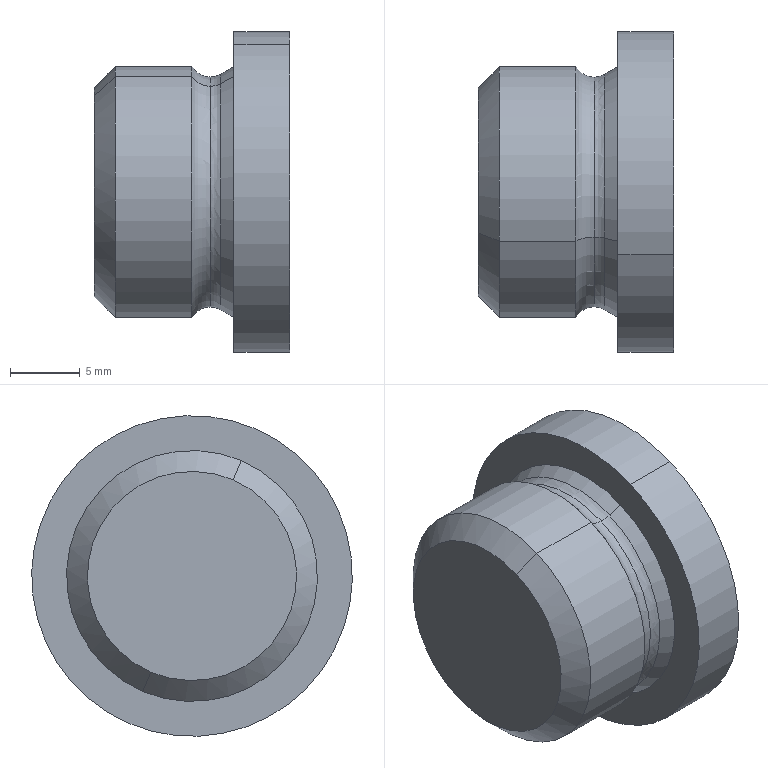Part | SolidWorks | features BaseBody 1 | 1 solid | 34 faces | box 14 x 23 x 23 mm | volume 3610 mm3 | plane 15 | cone 11 | torus 4 | cylinder 4 | commonest cylinder face diameters 18 x2 23 x2
STEP:
#1=CARTESIAN_POINT('',(329.849,223.125,-7.769));
#2=VERTEX_POINT('',#1);
#3=CARTESIAN_POINT('',(329.099,223.046,-7.584));
#4=VERTEX_POINT('',#3);
#5=CARTESIAN_POINT('',(329.099,223.636,-8.963));
#6=DIRECTION('',(0.,-0.9193,-0.3935));
#7=DIRECTION('',(0.,0.3935,-0.9193));
#8=AXIS2_PLACEMENT_3D('',#5,#6,#7);
#9=CIRCLE('',#8,1.5);
#10=EDGE_CURVE('',#2,#4,#9,.T.);
#11=ORIENTED_EDGE('',*,*,#10,.T.);
#12=CARTESIAN_POINT('',(329.099,216.554,7.584));
#13=VERTEX_POINT('',#12);
#14=CARTESIAN_POINT('',(329.099,219.8,0.));
#15=DIRECTION('',(1.,0.,0.));
#16=DIRECTION('',(0.,1.,0.));
#17=AXIS2_PLACEMENT_3D('',#14,#15,#16);
#18=CIRCLE('',#17,8.25);
#19=EDGE_CURVE('',#4,#13,#18,.T.);
#20=ORIENTED_EDGE('',*,*,#19,.T.);
#21=CARTESIAN_POINT('',(329.849,216.475,7.769));
#22=VERTEX_POINT('',#21);
#23=CARTESIAN_POINT('',(329.099,215.964,8.963));
#24=DIRECTION('',(0.,0.9193,0.3935));
#25=DIRECTION('',(0.,-0.3935,0.9193));
#26=AXIS2_PLACEMENT_3D('',#23,#24,#25);
#27=CIRCLE('',#26,1.5);
#28=EDGE_CURVE('',#22,#13,#27,.T.);
#29=ORIENTED_EDGE('',*,*,#28,.F.);
#30=CARTESIAN_POINT('',(329.849,219.8,0.));
#31=DIRECTION('',(1.,0.,0.));
#32=DIRECTION('',(0.,0.3935,-0.9193));
#33=AXIS2_PLACEMENT_3D('',#30,#31,#32);
#34=CIRCLE('',#33,8.451);
#35=EDGE_CURVE('',#2,#22,#34,.T.);
#36=ORIENTED_EDGE('',*,*,#35,.F.);
#37=EDGE_LOOP('',(#11,#20,#29,#36));
#38=FACE_OUTER_BOUND('',#37,.T.);
#39=CARTESIAN_POINT('',(329.099,219.8,0.));
#40=DIRECTION('',(1.,0.,0.));
#41=DIRECTION('',(0.,0.3935,-0.9193));
#42=AXIS2_PLACEMENT_3D('',#39,#40,#41);
#43=TOROIDAL_SURFACE('',#42,9.75,1.5);
#44=ADVANCED_FACE('',(#38),#43,.F.);
#45=ORIENTED_EDGE('',*,*,#28,.T.);
#46=CARTESIAN_POINT('',(329.099,219.8,0.));
#47=DIRECTION('',(1.,0.,0.));
#48=DIRECTION('',(0.,1.,0.));
#49=AXIS2_PLACEMENT_3D('',#46,#47,#48);
#50=CIRCLE('',#49,8.25);
#51=EDGE_CURVE('',#13,#4,#50,.T.);
#52=ORIENTED_EDGE('',*,*,#51,.T.);
#53=ORIENTED_EDGE('',*,*,#10,.F.);
#54=CARTESIAN_POINT('',(329.849,219.8,0.));
#55=DIRECTION('',(1.,0.,0.));
#56=DIRECTION('',(0.,0.3935,-0.9193));
#57=AXIS2_PLACEMENT_3D('',#54,#55,#56);
#58=CIRCLE('',#57,8.451);
#59=EDGE_CURVE('',#22,#2,#58,.T.);
#60=ORIENTED_EDGE('',*,*,#59,.F.);
#61=EDGE_LOOP('',(#45,#52,#53,#60));
#62=FACE_OUTER_BOUND('',#61,.T.);
#63=CARTESIAN_POINT('',(329.099,219.8,0.));
#64=DIRECTION('',(1.,0.,0.));
#65=DIRECTION('',(0.,0.3935,-0.9193));
#66=AXIS2_PLACEMENT_3D('',#63,#64,#65);
#67=TOROIDAL_SURFACE('',#66,9.75,1.5);
#68=ADVANCED_FACE('',(#62),#67,.F.);
#69=CARTESIAN_POINT('',(324.991,219.8,0.));
#70=VERTEX_POINT('',#69);
#71=CARTESIAN_POINT('',(327.3,221.374,-3.677));
#72=VERTEX_POINT('',#71);
#73=CARTESIAN_POINT('',(327.3,221.374,-3.677));
#74=DIRECTION('',(0.5,0.3408,-0.7962));
#75=VECTOR('',#74,1000.);
#76=LINE('',#73,#75);
#77=EDGE_CURVE('',#70,#72,#76,.T.);
#78=ORIENTED_EDGE('',*,*,#77,.F.);
#79=CARTESIAN_POINT('',(327.3,218.226,3.677));
#80=VERTEX_POINT('',#79);
#81=CARTESIAN_POINT('',(327.3,218.226,3.677));
#82=DIRECTION('',(0.5,-0.3408,0.7962));
#83=VECTOR('',#82,1000.);
#84=LINE('',#81,#83);
#85=EDGE_CURVE('',#70,#80,#84,.T.);
#86=ORIENTED_EDGE('',*,*,#85,.T.);
#87=CARTESIAN_POINT('',(327.3,215.825,0.4473));
#88=VERTEX_POINT('',#87);
#89=CARTESIAN_POINT('',(327.3,219.8,0.));
#90=DIRECTION('',(1.,0.,0.));
#91=DIRECTION('',(0.,0.3935,-0.9193));
#92=AXIS2_PLACEMENT_3D('',#89,#90,#91);
#93=CIRCLE('',#92,4.);
#94=EDGE_CURVE('',#80,#88,#93,.T.);
#95=ORIENTED_EDGE('',*,*,#94,.T.);
#96=CARTESIAN_POINT('',(327.3,217.38,-3.185));
#97=VERTEX_POINT('',#96);
#98=CARTESIAN_POINT('',(327.3,219.8,0.));
#99=DIRECTION('',(1.,0.,0.));
#100=DIRECTION('',(0.,0.3935,-0.9193));
#101=AXIS2_PLACEMENT_3D('',#98,#99,#100);
#102=CIRCLE('',#101,4.);
#103=EDGE_CURVE('',#88,#97,#102,.T.);
#104=ORIENTED_EDGE('',*,*,#103,.T.);
#105=CARTESIAN_POINT('',(327.3,219.8,0.));
#106=DIRECTION('',(1.,0.,0.));
#107=DIRECTION('',(0.,0.3935,-0.9193));
#108=AXIS2_PLACEMENT_3D('',#105,#106,#107);
#109=CIRCLE('',#108,4.);
#110=EDGE_CURVE('',#97,#72,#109,.T.);
#111=ORIENTED_EDGE('',*,*,#110,.T.);
#112=EDGE_LOOP('',(#78,#86,#95,#104,#111));
#113=FACE_OUTER_BOUND('',#112,.T.);
#114=CARTESIAN_POINT('',(327.3,219.8,0.));
#115=DIRECTION('',(1.,0.,0.));
#116=DIRECTION('',(0.,0.3935,-0.9193));
#117=AXIS2_PLACEMENT_3D('',#114,#115,#116);
#118=CONICAL_SURFACE('',#117,4.,1.047);
#119=ADVANCED_FACE('',(#113),#118,.F.);
#120=CARTESIAN_POINT('',(334.437,221.374,-3.677));
#121=VERTEX_POINT('',#120);
#122=CARTESIAN_POINT('',(334.8,223.515,-2.761));
#123=VERTEX_POINT('',#122);
#124=CARTESIAN_POINT('',(334.437,221.374,-3.677));
#125=CARTESIAN_POINT('',(334.437,221.736,-3.523));
#126=CARTESIAN_POINT('',(334.472,222.102,-3.366));
#127=CARTESIAN_POINT('',(334.599,222.818,-3.059));
#128=CARTESIAN_POINT('',(334.691,223.169,-2.909));
#129=CARTESIAN_POINT('',(334.8,223.515,-2.761));
#130=B_SPLINE_CURVE_WITH_KNOTS('',3,(#124,#125,#126,#127,#128,#129),.UNSPECIFIED.,.F.,.F.,(4,2,4),(0.006325,0.007503,0.008681),.UNSPECIFIED.);
#131=EDGE_CURVE('',#121,#123,#130,.T.);
#132=ORIENTED_EDGE('',*,*,#131,.F.);
#133=CARTESIAN_POINT('',(334.8,221.621,-4.255));
#134=VERTEX_POINT('',#133);
#135=CARTESIAN_POINT('',(334.8,221.621,-4.255));
#136=DIRECTION('',(0.5,0.3408,-0.7962));
#137=VECTOR('',#136,1000.);
#138=LINE('',#135,#137);
#139=EDGE_CURVE('',#121,#134,#138,.T.);
#140=ORIENTED_EDGE('',*,*,#139,.T.);
#141=CARTESIAN_POINT('',(334.8,219.8,0.));
#142=DIRECTION('',(1.,0.,0.));
#143=DIRECTION('',(0.,0.3935,-0.9193));
#144=AXIS2_PLACEMENT_3D('',#141,#142,#143);
#145=CIRCLE('',#144,4.628);
#146=EDGE_CURVE('',#134,#123,#145,.T.);
#147=ORIENTED_EDGE('',*,*,#146,.T.);
#148=EDGE_LOOP('',(#132,#140,#147));
#149=FACE_OUTER_BOUND('',#148,.T.);
#150=CARTESIAN_POINT('',(334.8,219.8,0.));
#151=DIRECTION('',(1.,0.,0.));
#152=DIRECTION('',(0.,0.3935,-0.9193));
#153=AXIS2_PLACEMENT_3D('',#150,#151,#152);
#154=CONICAL_SURFACE('',#153,4.628,1.047);
#155=ADVANCED_FACE('',(#149),#154,.F.);
#156=CARTESIAN_POINT('',(320.8,216.849,6.895));
#157=VERTEX_POINT('',#156);
#158=CARTESIAN_POINT('',(320.8,222.751,-6.895));
#159=VERTEX_POINT('',#158);
#160=CARTESIAN_POINT('',(320.8,219.8,0.));
#161=DIRECTION('',(-1.,0.,0.));
#162=DIRECTION('',(0.,-0.3935,0.9193));
#163=AXIS2_PLACEMENT_3D('',#160,#161,#162);
#164=CIRCLE('',#163,7.5);
#165=EDGE_CURVE('',#157,#159,#164,.T.);
#166=ORIENTED_EDGE('',*,*,#165,.F.);
#167=CARTESIAN_POINT('',(322.3,216.259,8.274));
#168=VERTEX_POINT('',#167);
#169=CARTESIAN_POINT('',(322.3,216.259,8.274));
#170=DIRECTION('',(0.7071,-0.2782,0.6501));
#171=VECTOR('',#170,1000.);
#172=LINE('',#169,#171);
#173=EDGE_CURVE('',#157,#168,#172,.T.);
#174=ORIENTED_EDGE('',*,*,#173,.T.);
#175=CARTESIAN_POINT('',(322.3,223.341,-8.274));
#176=VERTEX_POINT('',#175);
#177=CARTESIAN_POINT('',(322.3,219.8,0.));
#178=DIRECTION('',(1.,0.,0.));
#179=DIRECTION('',(0.,-0.3935,0.9193));
#180=AXIS2_PLACEMENT_3D('',#177,#178,#179);
#181=CIRCLE('',#180,9.);
#182=EDGE_CURVE('',#176,#168,#181,.T.);
#183=ORIENTED_EDGE('',*,*,#182,.F.);
#184=CARTESIAN_POINT('',(322.3,223.341,-8.274));
#185=DIRECTION('',(0.7071,0.2782,-0.6501));
#186=VECTOR('',#185,1000.);
#187=LINE('',#184,#186);
#188=EDGE_CURVE('',#159,#176,#187,.T.);
#189=ORIENTED_EDGE('',*,*,#188,.F.);
#190=EDGE_LOOP('',(#166,#174,#183,#189));
#191=FACE_OUTER_BOUND('',#190,.T.);
#192=CARTESIAN_POINT('',(322.3,219.8,0.));
#193=DIRECTION('',(1.,0.,0.));
#194=DIRECTION('',(0.,0.3935,-0.9193));
#195=AXIS2_PLACEMENT_3D('',#192,#193,#194);
#196=CONICAL_SURFACE('',#195,9.,0.7854);
#197=ADVANCED_FACE('',(#191),#196,.T.);
#198=ORIENTED_EDGE('',*,*,#182,.T.);
#199=CARTESIAN_POINT('',(327.8,216.259,8.274));
#200=VERTEX_POINT('',#199);
#201=CARTESIAN_POINT('',(337.921,216.259,8.274));
#202=DIRECTION('',(1.,0.,0.));
#203=VECTOR('',#202,1000.);
#204=LINE('',#201,#203);
#205=EDGE_CURVE('',#168,#200,#204,.T.);
#206=ORIENTED_EDGE('',*,*,#205,.T.);
#207=CARTESIAN_POINT('',(327.8,223.341,-8.274));
#208=VERTEX_POINT('',#207);
#209=CARTESIAN_POINT('',(327.8,219.8,0.));
#210=DIRECTION('',(1.,0.,0.));
#211=DIRECTION('',(0.,0.3935,-0.9193));
#212=AXIS2_PLACEMENT_3D('',#209,#210,#211);
#213=CIRCLE('',#212,9.);
#214=EDGE_CURVE('',#208,#200,#213,.T.);
#215=ORIENTED_EDGE('',*,*,#214,.F.);
#216=CARTESIAN_POINT('',(337.921,223.341,-8.274));
#217=DIRECTION('',(1.,0.,0.));
#218=VECTOR('',#217,1000.);
#219=LINE('',#216,#218);
#220=EDGE_CURVE('',#176,#208,#219,.T.);
#221=ORIENTED_EDGE('',*,*,#220,.F.);
#222=EDGE_LOOP('',(#198,#206,#215,#221));
#223=FACE_OUTER_BOUND('',#222,.T.);
#224=CARTESIAN_POINT('',(337.921,219.8,0.));
#225=DIRECTION('',(1.,0.,0.));
#226=DIRECTION('',(0.,0.3935,-0.9193));
#227=AXIS2_PLACEMENT_3D('',#224,#225,#226);
#228=CYLINDRICAL_SURFACE('',#227,9.);
#229=ADVANCED_FACE('',(#223),#228,.T.);
#230=ORIENTED_EDGE('',*,*,#51,.F.);
#231=CARTESIAN_POINT('',(329.099,215.964,8.963));
#232=DIRECTION('',(0.,0.9193,0.3935));
#233=DIRECTION('',(0.,-0.3935,0.9193));
#234=AXIS2_PLACEMENT_3D('',#231,#232,#233);
#235=CIRCLE('',#234,1.5);
#236=EDGE_CURVE('',#13,#200,#235,.T.);
#237=ORIENTED_EDGE('',*,*,#236,.T.);
#238=CARTESIAN_POINT('',(327.8,219.8,0.));
#239=DIRECTION('',(1.,0.,0.));
#240=DIRECTION('',(0.,0.3935,-0.9193));
#241=AXIS2_PLACEMENT_3D('',#238,#239,#240);
#242=CIRCLE('',#241,9.);
#243=EDGE_CURVE('',#200,#208,#242,.T.);
#244=ORIENTED_EDGE('',*,*,#243,.T.);
#245=CARTESIAN_POINT('',(329.099,223.636,-8.963));
#246=DIRECTION('',(0.,-0.9193,-0.3935));
#247=DIRECTION('',(0.,0.3935,-0.9193));
#248=AXIS2_PLACEMENT_3D('',#245,#246,#247);
#249=CIRCLE('',#248,1.5);
#250=EDGE_CURVE('',#4,#208,#249,.T.);
#251=ORIENTED_EDGE('',*,*,#250,.F.);
#252=EDGE_LOOP('',(#230,#237,#244,#251));
#253=FACE_OUTER_BOUND('',#252,.T.);
#254=CARTESIAN_POINT('',(329.099,219.8,0.));
#255=DIRECTION('',(1.,0.,0.));
#256=DIRECTION('',(0.,0.3935,-0.9193));
#257=AXIS2_PLACEMENT_3D('',#254,#255,#256);
#258=TOROIDAL_SURFACE('',#257,9.75,1.5);
#259=ADVANCED_FACE('',(#253),#258,.F.);
#260=ORIENTED_EDGE('',*,*,#35,.T.);
#261=CARTESIAN_POINT('',(330.8,216.259,8.274));
#262=VERTEX_POINT('',#261);
#263=CARTESIAN_POINT('',(330.8,216.259,8.274));
#264=DIRECTION('',(0.866,-0.1967,0.4597));
#265=VECTOR('',#264,1000.);
#266=LINE('',#263,#265);
#267=EDGE_CURVE('',#22,#262,#266,.T.);
#268=ORIENTED_EDGE('',*,*,#267,.T.);
#269=CARTESIAN_POINT('',(330.8,223.341,-8.274));
#270=VERTEX_POINT('',#269);
#271=CARTESIAN_POINT('',(330.8,219.8,0.));
#272=DIRECTION('',(1.,0.,0.));
#273=DIRECTION('',(0.,0.3935,-0.9193));
#274=AXIS2_PLACEMENT_3D('',#271,#272,#273);
#275=CIRCLE('',#274,9.);
#276=EDGE_CURVE('',#270,#262,#275,.T.);
#277=ORIENTED_EDGE('',*,*,#276,.F.);
#278=CARTESIAN_POINT('',(330.8,223.341,-8.274));
#279=DIRECTION('',(0.866,0.1967,-0.4597));
#280=VECTOR('',#279,1000.);
#281=LINE('',#278,#280);
#282=EDGE_CURVE('',#2,#270,#281,.T.);
#283=ORIENTED_EDGE('',*,*,#282,.F.);
#284=EDGE_LOOP('',(#260,#268,#277,#283));
#285=FACE_OUTER_BOUND('',#284,.T.);
#286=CARTESIAN_POINT('',(330.8,219.8,0.));
#287=DIRECTION('',(1.,0.,0.));
#288=DIRECTION('',(0.,0.3935,-0.9193));
#289=AXIS2_PLACEMENT_3D('',#286,#287,#288);
#290=CONICAL_SURFACE('',#289,9.,0.5236);
#291=ADVANCED_FACE('',(#285),#290,.T.);
#292=CARTESIAN_POINT('',(330.8,224.325,-10.572));
#293=VERTEX_POINT('',#292);
#294=CARTESIAN_POINT('',(330.8,215.275,10.572));
#295=VERTEX_POINT('',#294);
#296=CARTESIAN_POINT('',(330.8,219.8,0.));
#297=DIRECTION('',(1.,0.,0.));
#298=DIRECTION('',(0.,0.3935,-0.9193));
#299=AXIS2_PLACEMENT_3D('',#296,#297,#298);
#300=CIRCLE('',#299,11.5);
#301=EDGE_CURVE('',#293,#295,#300,.T.);
#302=ORIENTED_EDGE('',*,*,#301,.T.);
#303=CARTESIAN_POINT('',(334.8,215.275,10.572));
#304=VERTEX_POINT('',#303);
#305=CARTESIAN_POINT('',(337.921,215.275,10.572));
#306=DIRECTION('',(1.,0.,0.));
#307=VECTOR('',#306,1000.);
#308=LINE('',#305,#307);
#309=EDGE_CURVE('',#295,#304,#308,.T.);
#310=ORIENTED_EDGE('',*,*,#309,.T.);
#311=CARTESIAN_POINT('',(334.8,224.325,-10.572));
#312=VERTEX_POINT('',#311);
#313=CARTESIAN_POINT('',(334.8,219.8,0.));
#314=DIRECTION('',(1.,0.,0.));
#315=DIRECTION('',(0.,0.3935,-0.9193));
#316=AXIS2_PLACEMENT_3D('',#313,#314,#315);
#317=CIRCLE('',#316,11.5);
#318=EDGE_CURVE('',#312,#304,#317,.T.);
#319=ORIENTED_EDGE('',*,*,#318,.F.);
#320=CARTESIAN_POINT('',(337.921,224.325,-10.572));
#321=DIRECTION('',(1.,0.,0.));
#322=VECTOR('',#321,1000.);
#323=LINE('',#320,#322);
#324=EDGE_CURVE('',#293,#312,#323,.T.);
#325=ORIENTED_EDGE('',*,*,#324,.F.);
#326=EDGE_LOOP('',(#302,#310,#319,#325));
#327=FACE_OUTER_BOUND('',#326,.T.);
#328=CARTESIAN_POINT('',(337.921,219.8,0.));
#329=DIRECTION('',(1.,0.,0.));
#330=DIRECTION('',(0.,0.3935,-0.9193));
#331=AXIS2_PLACEMENT_3D('',#328,#329,#330);
#332=CYLINDRICAL_SURFACE('',#331,11.5);
#333=ADVANCED_FACE('',(#327),#332,.T.);
#334=CARTESIAN_POINT('',(327.3,220.367,4.594));
#335=VERTEX_POINT('',#334);
#336=CARTESIAN_POINT('',(327.3,216.085,2.761));
#337=DIRECTION('',(0.,-0.9193,-0.3935));
#338=VECTOR('',#337,1000.);
#339=LINE('',#336,#338);
#340=EDGE_CURVE('',#335,#80,#339,.T.);
#341=ORIENTED_EDGE('',*,*,#340,.T.);
#342=CARTESIAN_POINT('',(327.3,222.22,3.185));
#343=VERTEX_POINT('',#342);
#344=CARTESIAN_POINT('',(327.3,219.8,0.));
#345=DIRECTION('',(1.,0.,0.));
#346=DIRECTION('',(0.,0.3935,-0.9193));
#347=AXIS2_PLACEMENT_3D('',#344,#345,#346);
#348=CIRCLE('',#347,4.);
#349=EDGE_CURVE('',#343,#80,#348,.T.);
#350=ORIENTED_EDGE('',*,*,#349,.F.);
#351=CARTESIAN_POINT('',(327.3,220.367,4.594));
#352=DIRECTION('',(0.,-0.7961,0.6051));
#353=VECTOR('',#352,1000.);
#354=LINE('',#351,#353);
#355=EDGE_CURVE('',#343,#335,#354,.T.);
#356=ORIENTED_EDGE('',*,*,#355,.T.);
#357=EDGE_LOOP('',(#341,#350,#356));
#358=FACE_OUTER_BOUND('',#357,.T.);
#359=CARTESIAN_POINT('',(327.3,224.543,6.381));
#360=DIRECTION('',(-1.,0.,0.));
#361=DIRECTION('',(0.,-0.3935,0.9193));
#362=AXIS2_PLACEMENT_3D('',#359,#360,#361);
#363=PLANE('',#362);
#364=ADVANCED_FACE('',(#358),#363,.F.);
#365=CARTESIAN_POINT('',(327.3,224.029,1.81));
#366=VERTEX_POINT('',#365);
#367=CARTESIAN_POINT('',(327.3,220.367,4.594));
#368=DIRECTION('',(0.,-0.7961,0.6051));
#369=VECTOR('',#368,1000.);
#370=LINE('',#367,#369);
#371=EDGE_CURVE('',#366,#343,#370,.T.);
#372=ORIENTED_EDGE('',*,*,#371,.T.);
#373=CARTESIAN_POINT('',(327.3,223.775,-0.4473));
#374=VERTEX_POINT('',#373);
#375=CARTESIAN_POINT('',(327.3,219.8,0.));
#376=DIRECTION('',(1.,0.,0.));
#377=DIRECTION('',(0.,0.3935,-0.9193));
#378=AXIS2_PLACEMENT_3D('',#375,#376,#377);
#379=CIRCLE('',#378,4.);
#380=EDGE_CURVE('',#374,#343,#379,.T.);
#381=ORIENTED_EDGE('',*,*,#380,.F.);
#382=CARTESIAN_POINT('',(327.3,223.515,-2.761));
#383=DIRECTION('',(0.,0.1118,0.9937));
#384=VECTOR('',#383,1000.);
#385=LINE('',#382,#384);
#386=EDGE_CURVE('',#374,#366,#385,.T.);
#387=ORIENTED_EDGE('',*,*,#386,.T.);
#388=EDGE_LOOP('',(#372,#381,#387));
#389=FACE_OUTER_BOUND('',#388,.T.);
#390=CARTESIAN_POINT('',(327.3,224.543,6.381));
#391=DIRECTION('',(-1.,0.,0.));
#392=DIRECTION('',(0.,-0.3935,0.9193));
#393=AXIS2_PLACEMENT_3D('',#390,#391,#392);
#394=PLANE('',#393);
#395=ADVANCED_FACE('',(#389),#394,.F.);
#396=CARTESIAN_POINT('',(327.3,223.515,-2.761));
#397=VERTEX_POINT('',#396);
#398=CARTESIAN_POINT('',(327.3,223.515,-2.761));
#399=DIRECTION('',(0.,0.1118,0.9937));
#400=VECTOR('',#399,1000.);
#401=LINE('',#398,#400);
#402=EDGE_CURVE('',#397,#374,#401,.T.);
#403=ORIENTED_EDGE('',*,*,#402,.T.);
#404=CARTESIAN_POINT('',(327.3,219.8,0.));
#405=DIRECTION('',(1.,0.,0.));
#406=DIRECTION('',(0.,0.3935,-0.9193));
#407=AXIS2_PLACEMENT_3D('',#404,#405,#406);
#408=CIRCLE('',#407,4.);
#409=EDGE_CURVE('',#72,#374,#408,.T.);
#410=ORIENTED_EDGE('',*,*,#409,.F.);
#411=CARTESIAN_POINT('',(327.3,219.233,-4.594));
#412=DIRECTION('',(0.,0.9193,0.3935));
#413=VECTOR('',#412,1000.);
#414=LINE('',#411,#413);
#415=EDGE_CURVE('',#72,#397,#414,.T.);
#416=ORIENTED_EDGE('',*,*,#415,.T.);
#417=EDGE_LOOP('',(#403,#410,#416));
#418=FACE_OUTER_BOUND('',#417,.T.);
#419=CARTESIAN_POINT('',(327.3,224.543,6.381));
#420=DIRECTION('',(-1.,0.,0.));
#421=DIRECTION('',(0.,-0.3935,0.9193));
#422=AXIS2_PLACEMENT_3D('',#419,#420,#421);
#423=PLANE('',#422);
#424=ADVANCED_FACE('',(#418),#423,.F.);
#425=CARTESIAN_POINT('',(327.3,219.233,-4.594));
#426=VERTEX_POINT('',#425);
#427=CARTESIAN_POINT('',(327.3,219.233,-4.594));
#428=DIRECTION('',(0.,0.9193,0.3935));
#429=VECTOR('',#428,1000.);
#430=LINE('',#427,#429);
#431=EDGE_CURVE('',#426,#72,#430,.T.);
#432=ORIENTED_EDGE('',*,*,#431,.T.);
#433=ORIENTED_EDGE('',*,*,#110,.F.);
#434=CARTESIAN_POINT('',(327.3,219.233,-4.594));
#435=DIRECTION('',(0.,0.7961,-0.6051));
#436=VECTOR('',#435,1000.);
#437=LINE('',#434,#436);
#438=EDGE_CURVE('',#97,#426,#437,.T.);
#439=ORIENTED_EDGE('',*,*,#438,.T.);
#440=EDGE_LOOP('',(#432,#433,#439));
#441=FACE_OUTER_BOUND('',#440,.T.);
#442=CARTESIAN_POINT('',(327.3,224.543,6.381));
#443=DIRECTION('',(-1.,0.,0.));
#444=DIRECTION('',(0.,-0.3935,0.9193));
#445=AXIS2_PLACEMENT_3D('',#442,#443,#444);
#446=PLANE('',#445);
#447=ADVANCED_FACE('',(#441),#446,.F.);
#448=CARTESIAN_POINT('',(327.3,215.571,-1.81));
#449=VERTEX_POINT('',#448);
#450=CARTESIAN_POINT('',(327.3,219.233,-4.594));
#451=DIRECTION('',(0.,0.7961,-0.6051));
#452=VECTOR('',#451,1000.);
#453=LINE('',#450,#452);
#454=EDGE_CURVE('',#449,#97,#453,.T.);
#455=ORIENTED_EDGE('',*,*,#454,.T.);
#456=ORIENTED_EDGE('',*,*,#103,.F.);
#457=CARTESIAN_POINT('',(327.3,216.085,2.761));
#458=DIRECTION('',(0.,-0.1118,-0.9937));
#459=VECTOR('',#458,1000.);
#460=LINE('',#457,#459);
#461=EDGE_CURVE('',#88,#449,#460,.T.);
#462=ORIENTED_EDGE('',*,*,#461,.T.);
#463=EDGE_LOOP('',(#455,#456,#462));
#464=FACE_OUTER_BOUND('',#463,.T.);
#465=CARTESIAN_POINT('',(327.3,224.543,6.381));
#466=DIRECTION('',(-1.,0.,0.));
#467=DIRECTION('',(0.,-0.3935,0.9193));
#468=AXIS2_PLACEMENT_3D('',#465,#466,#467);
#469=PLANE('',#468);
#470=ADVANCED_FACE('',(#464),#469,.F.);
#471=CARTESIAN_POINT('',(334.8,220.367,4.594));
#472=VERTEX_POINT('',#471);
#473=CARTESIAN_POINT('',(334.8,219.8,0.));
#474=DIRECTION('',(1.,0.,0.));
#475=DIRECTION('',(0.,0.3935,-0.9193));
#476=AXIS2_PLACEMENT_3D('',#473,#474,#475);
#477=CIRCLE('',#476,4.628);
#478=EDGE_CURVE('',#123,#472,#477,.T.);
#479=ORIENTED_EDGE('',*,*,#478,.F.);
#480=ORIENTED_EDGE('',*,*,#146,.F.);
#481=CARTESIAN_POINT('',(334.8,219.233,-4.594));
#482=VERTEX_POINT('',#481);
#483=CARTESIAN_POINT('',(334.8,219.8,0.));
#484=DIRECTION('',(1.,0.,0.));
#485=DIRECTION('',(0.,0.3935,-0.9193));
#486=AXIS2_PLACEMENT_3D('',#483,#484,#485);
#487=CIRCLE('',#486,4.628);
#488=EDGE_CURVE('',#482,#134,#487,.T.);
#489=ORIENTED_EDGE('',*,*,#488,.F.);
#490=CARTESIAN_POINT('',(334.8,216.085,2.761));
#491=VERTEX_POINT('',#490);
#492=CARTESIAN_POINT('',(334.8,219.8,0.));
#493=DIRECTION('',(1.,0.,0.));
#494=DIRECTION('',(0.,0.3935,-0.9193));
#495=AXIS2_PLACEMENT_3D('',#492,#493,#494);
#496=CIRCLE('',#495,4.628);
#497=EDGE_CURVE('',#491,#482,#496,.T.);
#498=ORIENTED_EDGE('',*,*,#497,.F.);
#499=CARTESIAN_POINT('',(334.8,219.8,0.));
#500=DIRECTION('',(1.,0.,0.));
#501=DIRECTION('',(0.,0.3935,-0.9193));
#502=AXIS2_PLACEMENT_3D('',#499,#500,#501);
#503=CIRCLE('',#502,4.628);
#504=EDGE_CURVE('',#472,#491,#503,.T.);
#505=ORIENTED_EDGE('',*,*,#504,.F.);
#506=EDGE_LOOP('',(#479,#480,#489,#498,#505));
#507=FACE_BOUND('',#506,.T.);
#508=ORIENTED_EDGE('',*,*,#318,.T.);
#509=CARTESIAN_POINT('',(334.8,219.8,0.));
#510=DIRECTION('',(1.,0.,0.));
#511=DIRECTION('',(0.,0.3935,-0.9193));
#512=AXIS2_PLACEMENT_3D('',#509,#510,#511);
#513=CIRCLE('',#512,11.5);
#514=EDGE_CURVE('',#304,#312,#513,.T.);
#515=ORIENTED_EDGE('',*,*,#514,.T.);
#516=EDGE_LOOP('',(#508,#515));
#517=FACE_OUTER_BOUND('',#516,.T.);
#518=CARTESIAN_POINT('',(334.8,219.8,0.));
#519=DIRECTION('',(1.,0.,0.));
#520=DIRECTION('',(0.,0.3935,-0.9193));
#521=AXIS2_PLACEMENT_3D('',#518,#519,#520);
#522=PLANE('',#521);
#523=ADVANCED_FACE('',(#507,#517),#522,.T.);
#524=ORIENTED_EDGE('',*,*,#309,.F.);
#525=CARTESIAN_POINT('',(330.8,219.8,0.));
#526=DIRECTION('',(1.,0.,0.));
#527=DIRECTION('',(0.,0.3935,-0.9193));
#528=AXIS2_PLACEMENT_3D('',#525,#526,#527);
#529=CIRCLE('',#528,11.5);
#530=EDGE_CURVE('',#295,#293,#529,.T.);
#531=ORIENTED_EDGE('',*,*,#530,.T.);
#532=ORIENTED_EDGE('',*,*,#324,.T.);
#533=ORIENTED_EDGE('',*,*,#514,.F.);
#534=EDGE_LOOP('',(#524,#531,#532,#533));
#535=FACE_OUTER_BOUND('',#534,.T.);
#536=CARTESIAN_POINT('',(337.921,219.8,0.));
#537=DIRECTION('',(1.,0.,0.));
#538=DIRECTION('',(0.,0.3935,-0.9193));
#539=AXIS2_PLACEMENT_3D('',#536,#537,#538);
#540=CYLINDRICAL_SURFACE('',#539,11.5);
#541=ADVANCED_FACE('',(#535),#540,.T.);
#542=ORIENTED_EDGE('',*,*,#276,.T.);
#543=CARTESIAN_POINT('',(330.8,219.8,0.));
#544=DIRECTION('',(1.,0.,0.));
#545=DIRECTION('',(0.,0.3935,-0.9193));
#546=AXIS2_PLACEMENT_3D('',#543,#544,#545);
#547=CIRCLE('',#546,9.);
#548=EDGE_CURVE('',#262,#270,#547,.T.);
#549=ORIENTED_EDGE('',*,*,#548,.T.);
#550=EDGE_LOOP('',(#542,#549));
#551=FACE_BOUND('',#550,.T.);
#552=ORIENTED_EDGE('',*,*,#301,.F.);
#553=ORIENTED_EDGE('',*,*,#530,.F.);
#554=EDGE_LOOP('',(#552,#553));
#555=FACE_OUTER_BOUND('',#554,.T.);
#556=CARTESIAN_POINT('',(330.8,230.372,4.525));
#557=DIRECTION('',(-1.,0.,0.));
#558=DIRECTION('',(0.,-0.3935,0.9193));
#559=AXIS2_PLACEMENT_3D('',#556,#557,#558);
#560=PLANE('',#559);
#561=ADVANCED_FACE('',(#551,#555),#560,.T.);
#562=ORIENTED_EDGE('',*,*,#267,.F.);
#563=ORIENTED_EDGE('',*,*,#59,.T.);
#564=ORIENTED_EDGE('',*,*,#282,.T.);
#565=ORIENTED_EDGE('',*,*,#548,.F.);
#566=EDGE_LOOP('',(#562,#563,#564,#565));
#567=FACE_OUTER_BOUND('',#566,.T.);
#568=CARTESIAN_POINT('',(330.8,219.8,0.));
#569=DIRECTION('',(1.,0.,0.));
#570=DIRECTION('',(0.,0.3935,-0.9193));
#571=AXIS2_PLACEMENT_3D('',#568,#569,#570);
#572=CONICAL_SURFACE('',#571,9.,0.5236);
#573=ADVANCED_FACE('',(#567),#572,.T.);
#574=ORIENTED_EDGE('',*,*,#19,.F.);
#575=ORIENTED_EDGE('',*,*,#250,.T.);
#576=ORIENTED_EDGE('',*,*,#214,.T.);
#577=ORIENTED_EDGE('',*,*,#236,.F.);
#578=EDGE_LOOP('',(#574,#575,#576,#577));
#579=FACE_OUTER_BOUND('',#578,.T.);
#580=CARTESIAN_POINT('',(329.099,219.8,0.));
#581=DIRECTION('',(1.,0.,0.));
#582=DIRECTION('',(0.,0.3935,-0.9193));
#583=AXIS2_PLACEMENT_3D('',#580,#581,#582);
#584=TOROIDAL_SURFACE('',#583,9.75,1.5);
#585=ADVANCED_FACE('',(#579),#584,.F.);
#586=ORIENTED_EDGE('',*,*,#205,.F.);
#587=CARTESIAN_POINT('',(322.3,219.8,0.));
#588=DIRECTION('',(1.,0.,0.));
#589=DIRECTION('',(0.,-0.3935,0.9193));
#590=AXIS2_PLACEMENT_3D('',#587,#588,#589);
#591=CIRCLE('',#590,9.);
#592=EDGE_CURVE('',#168,#176,#591,.T.);
#593=ORIENTED_EDGE('',*,*,#592,.T.);
#594=ORIENTED_EDGE('',*,*,#220,.T.);
#595=ORIENTED_EDGE('',*,*,#243,.F.);
#596=EDGE_LOOP('',(#586,#593,#594,#595));
#597=FACE_OUTER_BOUND('',#596,.T.);
#598=CARTESIAN_POINT('',(337.921,219.8,0.));
#599=DIRECTION('',(1.,0.,0.));
#600=DIRECTION('',(0.,0.3935,-0.9193));
#601=AXIS2_PLACEMENT_3D('',#598,#599,#600);
#602=CYLINDRICAL_SURFACE('',#601,9.);
#603=ADVANCED_FACE('',(#597),#602,.T.);
#604=CARTESIAN_POINT('',(320.8,219.8,0.));
#605=DIRECTION('',(-1.,0.,0.));
#606=DIRECTION('',(0.,-0.3935,0.9193));
#607=AXIS2_PLACEMENT_3D('',#604,#605,#606);
#608=CIRCLE('',#607,7.5);
#609=EDGE_CURVE('',#159,#157,#608,.T.);
#610=ORIENTED_EDGE('',*,*,#609,.T.);
#611=ORIENTED_EDGE('',*,*,#165,.T.);
#612=EDGE_LOOP('',(#610,#611));
#613=FACE_OUTER_BOUND('',#612,.T.);
#614=CARTESIAN_POINT('',(320.8,228.074,3.541));
#615=DIRECTION('',(-1.,0.,0.));
#616=DIRECTION('',(0.,-0.3935,0.9193));
#617=AXIS2_PLACEMENT_3D('',#614,#615,#616);
#618=PLANE('',#617);
#619=ADVANCED_FACE('',(#613),#618,.T.);
#620=ORIENTED_EDGE('',*,*,#173,.F.);
#621=ORIENTED_EDGE('',*,*,#609,.F.);
#622=ORIENTED_EDGE('',*,*,#188,.T.);
#623=ORIENTED_EDGE('',*,*,#592,.F.);
#624=EDGE_LOOP('',(#620,#621,#622,#623));
#625=FACE_OUTER_BOUND('',#624,.T.);
#626=CARTESIAN_POINT('',(322.3,219.8,0.));
#627=DIRECTION('',(1.,0.,0.));
#628=DIRECTION('',(0.,0.3935,-0.9193));
#629=AXIS2_PLACEMENT_3D('',#626,#627,#628);
#630=CONICAL_SURFACE('',#629,9.,0.7854);
#631=ADVANCED_FACE('',(#625),#630,.T.);
#632=ORIENTED_EDGE('',*,*,#478,.T.);
#633=CARTESIAN_POINT('',(334.784,224.029,1.81));
#634=VERTEX_POINT('',#633);
#635=CARTESIAN_POINT('',(334.784,224.029,1.81));
#636=CARTESIAN_POINT('',(334.569,223.43,2.265));
#637=CARTESIAN_POINT('',(334.434,222.823,2.727));
#638=CARTESIAN_POINT('',(334.439,221.889,3.436));
#639=CARTESIAN_POINT('',(334.474,221.578,3.673));
#640=CARTESIAN_POINT('',(334.6,220.968,4.137));
#641=CARTESIAN_POINT('',(334.691,220.666,4.366));
#642=CARTESIAN_POINT('',(334.8,220.367,4.594));
#643=B_SPLINE_CURVE_WITH_KNOTS('',3,(#635,#636,#637,#638,#639,#640,#641,#642),.UNSPECIFIED.,.F.,.F.,(4,2,2,4),(0.000000237,0.002323,0.003484,0.004645),.UNSPECIFIED.);
#644=EDGE_CURVE('',#634,#472,#643,.T.);
#645=ORIENTED_EDGE('',*,*,#644,.F.);
#646=CARTESIAN_POINT('',(334.8,223.515,-2.761));
#647=CARTESIAN_POINT('',(334.582,223.598,-2.015));
#648=CARTESIAN_POINT('',(334.441,223.684,-1.258));
#649=CARTESIAN_POINT('',(334.435,223.815,-0.09279));
#650=CARTESIAN_POINT('',(334.468,223.859,0.2958));
#651=CARTESIAN_POINT('',(334.588,223.944,1.059));
#652=CARTESIAN_POINT('',(334.676,223.987,1.436));
#653=CARTESIAN_POINT('',(334.784,224.029,1.81));
#654=B_SPLINE_CURVE_WITH_KNOTS('',3,(#646,#647,#648,#649,#650,#651,#652,#653),.UNSPECIFIED.,.F.,.F.,(4,2,2,4),(0.000000237,0.002323,0.003484,0.004645),.UNSPECIFIED.);
#655=EDGE_CURVE('',#123,#634,#654,.T.);
#656=ORIENTED_EDGE('',*,*,#655,.F.);
#657=EDGE_LOOP('',(#632,#645,#656));
#658=FACE_OUTER_BOUND('',#657,.T.);
#659=CARTESIAN_POINT('',(334.8,219.8,0.));
#660=DIRECTION('',(1.,0.,0.));
#661=DIRECTION('',(0.,0.3935,-0.9193));
#662=AXIS2_PLACEMENT_3D('',#659,#660,#661);
#663=CONICAL_SURFACE('',#662,4.628,1.047);
#664=ADVANCED_FACE('',(#658),#663,.F.);
#665=ORIENTED_EDGE('',*,*,#504,.T.);
#666=CARTESIAN_POINT('',(334.8,220.367,4.594));
#667=CARTESIAN_POINT('',(334.691,220.021,4.445));
#668=CARTESIAN_POINT('',(334.6,219.67,4.295));
#669=CARTESIAN_POINT('',(334.472,218.955,3.989));
#670=CARTESIAN_POINT('',(334.437,218.588,3.832));
#671=CARTESIAN_POINT('',(334.437,217.865,3.523));
#672=CARTESIAN_POINT('',(334.471,217.505,3.369));
#673=CARTESIAN_POINT('',(334.598,216.79,3.063));
#674=CARTESIAN_POINT('',(334.69,216.433,2.91));
#675=CARTESIAN_POINT('',(334.8,216.085,2.761));
#676=B_SPLINE_CURVE_WITH_KNOTS('',3,(#666,#667,#668,#669,#670,#671,#672,#673,#674,#675),.UNSPECIFIED.,.F.,.F.,(4,2,2,2,4),(0.001817,0.002992,0.004167,0.005343,0.006518),.UNSPECIFIED.);
#677=EDGE_CURVE('',#472,#491,#676,.T.);
#678=ORIENTED_EDGE('',*,*,#677,.F.);
#679=EDGE_LOOP('',(#665,#678));
#680=FACE_OUTER_BOUND('',#679,.T.);
#681=CARTESIAN_POINT('',(334.8,219.8,0.));
#682=DIRECTION('',(1.,0.,0.));
#683=DIRECTION('',(0.,0.3935,-0.9193));
#684=AXIS2_PLACEMENT_3D('',#681,#682,#683);
#685=CONICAL_SURFACE('',#684,4.628,1.047);
#686=ADVANCED_FACE('',(#680),#685,.F.);
#687=CARTESIAN_POINT('',(334.784,215.571,-1.81));
#688=VERTEX_POINT('',#687);
#689=CARTESIAN_POINT('',(334.8,216.085,2.761));
#690=CARTESIAN_POINT('',(334.582,216.002,2.015));
#691=CARTESIAN_POINT('',(334.441,215.916,1.258));
#692=CARTESIAN_POINT('',(334.435,215.785,0.09279));
#693=CARTESIAN_POINT('',(334.468,215.741,-0.2958));
#694=CARTESIAN_POINT('',(334.588,215.656,-1.059));
#695=CARTESIAN_POINT('',(334.676,215.613,-1.436));
#696=CARTESIAN_POINT('',(334.784,215.571,-1.81));
#697=B_SPLINE_CURVE_WITH_KNOTS('',3,(#689,#690,#691,#692,#693,#694,#695,#696),.UNSPECIFIED.,.F.,.F.,(4,2,2,4),(0.000000237,0.002323,0.003484,0.004645),.UNSPECIFIED.);
#698=EDGE_CURVE('',#491,#688,#697,.T.);
#699=ORIENTED_EDGE('',*,*,#698,.F.);
#700=ORIENTED_EDGE('',*,*,#497,.T.);
#701=CARTESIAN_POINT('',(334.784,215.571,-1.81));
#702=CARTESIAN_POINT('',(334.569,216.17,-2.265));
#703=CARTESIAN_POINT('',(334.434,216.777,-2.727));
#704=CARTESIAN_POINT('',(334.439,217.711,-3.436));
#705=CARTESIAN_POINT('',(334.474,218.022,-3.673));
#706=CARTESIAN_POINT('',(334.6,218.632,-4.137));
#707=CARTESIAN_POINT('',(334.691,218.934,-4.366));
#708=CARTESIAN_POINT('',(334.8,219.233,-4.594));
#709=B_SPLINE_CURVE_WITH_KNOTS('',3,(#701,#702,#703,#704,#705,#706,#707,#708),.UNSPECIFIED.,.F.,.F.,(4,2,2,4),(0.000000237,0.002323,0.003484,0.004645),.UNSPECIFIED.);
#710=EDGE_CURVE('',#688,#482,#709,.T.);
#711=ORIENTED_EDGE('',*,*,#710,.F.);
#712=EDGE_LOOP('',(#699,#700,#711));
#713=FACE_OUTER_BOUND('',#712,.T.);
#714=CARTESIAN_POINT('',(334.8,219.8,0.));
#715=DIRECTION('',(1.,0.,0.));
#716=DIRECTION('',(0.,0.3935,-0.9193));
#717=AXIS2_PLACEMENT_3D('',#714,#715,#716);
#718=CONICAL_SURFACE('',#717,4.628,1.047);
#719=ADVANCED_FACE('',(#713),#718,.F.);
#720=ORIENTED_EDGE('',*,*,#139,.F.);
#721=CARTESIAN_POINT('',(334.8,219.233,-4.594));
#722=CARTESIAN_POINT('',(334.69,219.581,-4.445));
#723=CARTESIAN_POINT('',(334.598,219.937,-4.292));
#724=CARTESIAN_POINT('',(334.471,220.653,-3.986));
#725=CARTESIAN_POINT('',(334.437,221.012,-3.832));
#726=CARTESIAN_POINT('',(334.437,221.374,-3.677));
#727=B_SPLINE_CURVE_WITH_KNOTS('',3,(#721,#722,#723,#724,#725,#726),.UNSPECIFIED.,.F.,.F.,(4,2,4),(0.003971,0.005148,0.006325),.UNSPECIFIED.);
#728=EDGE_CURVE('',#482,#121,#727,.T.);
#729=ORIENTED_EDGE('',*,*,#728,.F.);
#730=ORIENTED_EDGE('',*,*,#488,.T.);
#731=EDGE_LOOP('',(#720,#729,#730));
#732=FACE_OUTER_BOUND('',#731,.T.);
#733=CARTESIAN_POINT('',(334.8,219.8,0.));
#734=DIRECTION('',(1.,0.,0.));
#735=DIRECTION('',(0.,0.3935,-0.9193));
#736=AXIS2_PLACEMENT_3D('',#733,#734,#735);
#737=CONICAL_SURFACE('',#736,4.628,1.047);
#738=ADVANCED_FACE('',(#732),#737,.F.);
#739=CARTESIAN_POINT('',(327.3,216.085,2.761));
#740=VERTEX_POINT('',#739);
#741=CARTESIAN_POINT('',(327.3,216.085,2.761));
#742=DIRECTION('',(0.,-0.1118,-0.9937));
#743=VECTOR('',#742,1000.);
#744=LINE('',#741,#743);
#745=EDGE_CURVE('',#740,#88,#744,.T.);
#746=ORIENTED_EDGE('',*,*,#745,.T.);
#747=ORIENTED_EDGE('',*,*,#94,.F.);
#748=CARTESIAN_POINT('',(327.3,216.085,2.761));
#749=DIRECTION('',(0.,-0.9193,-0.3935));
#750=VECTOR('',#749,1000.);
#751=LINE('',#748,#750);
#752=EDGE_CURVE('',#80,#740,#751,.T.);
#753=ORIENTED_EDGE('',*,*,#752,.T.);
#754=EDGE_LOOP('',(#746,#747,#753));
#755=FACE_OUTER_BOUND('',#754,.T.);
#756=CARTESIAN_POINT('',(327.3,224.543,6.381));
#757=DIRECTION('',(-1.,0.,0.));
#758=DIRECTION('',(0.,-0.3935,0.9193));
#759=AXIS2_PLACEMENT_3D('',#756,#757,#758);
#760=PLANE('',#759);
#761=ADVANCED_FACE('',(#755),#760,.F.);
#762=CARTESIAN_POINT('',(327.3,224.029,1.81));
#763=DIRECTION('',(1.,0.,0.));
#764=VECTOR('',#763,1000.);
#765=LINE('',#762,#764);
#766=EDGE_CURVE('',#366,#634,#765,.T.);
#767=ORIENTED_EDGE('',*,*,#766,.T.);
#768=ORIENTED_EDGE('',*,*,#644,.T.);
#769=CARTESIAN_POINT('',(327.3,220.367,4.594));
#770=DIRECTION('',(1.,0.,0.));
#771=VECTOR('',#770,1000.);
#772=LINE('',#769,#771);
#773=EDGE_CURVE('',#335,#472,#772,.T.);
#774=ORIENTED_EDGE('',*,*,#773,.F.);
#775=ORIENTED_EDGE('',*,*,#355,.F.);
#776=ORIENTED_EDGE('',*,*,#371,.F.);
#777=EDGE_LOOP('',(#767,#768,#774,#775,#776));
#778=FACE_OUTER_BOUND('',#777,.T.);
#779=CARTESIAN_POINT('',(327.3,220.367,4.594));
#780=DIRECTION('',(0.,0.6051,0.7961));
#781=DIRECTION('',(0.,0.7961,-0.6051));
#782=AXIS2_PLACEMENT_3D('',#779,#780,#781);
#783=PLANE('',#782);
#784=ADVANCED_FACE('',(#778),#783,.F.);
#785=ORIENTED_EDGE('',*,*,#773,.T.);
#786=ORIENTED_EDGE('',*,*,#677,.T.);
#787=CARTESIAN_POINT('',(327.3,216.085,2.761));
#788=DIRECTION('',(1.,0.,0.));
#789=VECTOR('',#788,1000.);
#790=LINE('',#787,#789);
#791=EDGE_CURVE('',#740,#491,#790,.T.);
#792=ORIENTED_EDGE('',*,*,#791,.F.);
#793=ORIENTED_EDGE('',*,*,#752,.F.);
#794=ORIENTED_EDGE('',*,*,#340,.F.);
#795=EDGE_LOOP('',(#785,#786,#792,#793,#794));
#796=FACE_OUTER_BOUND('',#795,.T.);
#797=CARTESIAN_POINT('',(327.3,216.085,2.761));
#798=DIRECTION('',(0.,-0.3935,0.9193));
#799=DIRECTION('',(0.,0.9193,0.3935));
#800=AXIS2_PLACEMENT_3D('',#797,#798,#799);
#801=PLANE('',#800);
#802=ADVANCED_FACE('',(#796),#801,.F.);
#803=ORIENTED_EDGE('',*,*,#791,.T.);
#804=ORIENTED_EDGE('',*,*,#698,.T.);
#805=CARTESIAN_POINT('',(327.3,215.571,-1.81));
#806=DIRECTION('',(1.,0.,0.));
#807=VECTOR('',#806,1000.);
#808=LINE('',#805,#807);
#809=EDGE_CURVE('',#449,#688,#808,.T.);
#810=ORIENTED_EDGE('',*,*,#809,.F.);
#811=ORIENTED_EDGE('',*,*,#461,.F.);
#812=ORIENTED_EDGE('',*,*,#745,.F.);
#813=EDGE_LOOP('',(#803,#804,#810,#811,#812));
#814=FACE_OUTER_BOUND('',#813,.T.);
#815=CARTESIAN_POINT('',(327.3,216.085,2.761));
#816=DIRECTION('',(0.,-0.9937,0.1118));
#817=DIRECTION('',(0.,0.1118,0.9937));
#818=AXIS2_PLACEMENT_3D('',#815,#816,#817);
#819=PLANE('',#818);
#820=ADVANCED_FACE('',(#814),#819,.F.);
#821=ORIENTED_EDGE('',*,*,#809,.T.);
#822=ORIENTED_EDGE('',*,*,#710,.T.);
#823=CARTESIAN_POINT('',(327.3,219.233,-4.594));
#824=DIRECTION('',(1.,0.,0.));
#825=VECTOR('',#824,1000.);
#826=LINE('',#823,#825);
#827=EDGE_CURVE('',#426,#482,#826,.T.);
#828=ORIENTED_EDGE('',*,*,#827,.F.);
#829=ORIENTED_EDGE('',*,*,#438,.F.);
#830=ORIENTED_EDGE('',*,*,#454,.F.);
#831=EDGE_LOOP('',(#821,#822,#828,#829,#830));
#832=FACE_OUTER_BOUND('',#831,.T.);
#833=CARTESIAN_POINT('',(327.3,219.233,-4.594));
#834=DIRECTION('',(0.,-0.6051,-0.7961));
#835=DIRECTION('',(0.,-0.7961,0.6051));
#836=AXIS2_PLACEMENT_3D('',#833,#834,#835);
#837=PLANE('',#836);
#838=ADVANCED_FACE('',(#832),#837,.F.);
#839=ORIENTED_EDGE('',*,*,#827,.T.);
#840=ORIENTED_EDGE('',*,*,#728,.T.);
#841=ORIENTED_EDGE('',*,*,#131,.T.);
#842=CARTESIAN_POINT('',(327.3,223.515,-2.761));
#843=DIRECTION('',(1.,0.,0.));
#844=VECTOR('',#843,1000.);
#845=LINE('',#842,#844);
#846=EDGE_CURVE('',#397,#123,#845,.T.);
#847=ORIENTED_EDGE('',*,*,#846,.F.);
#848=ORIENTED_EDGE('',*,*,#415,.F.);
#849=ORIENTED_EDGE('',*,*,#431,.F.);
#850=EDGE_LOOP('',(#839,#840,#841,#847,#848,#849));
#851=FACE_OUTER_BOUND('',#850,.T.);
#852=CARTESIAN_POINT('',(327.3,219.233,-4.594));
#853=DIRECTION('',(0.,0.3935,-0.9193));
#854=DIRECTION('',(0.,-0.9193,-0.3935));
#855=AXIS2_PLACEMENT_3D('',#852,#853,#854);
#856=PLANE('',#855);
#857=ADVANCED_FACE('',(#851),#856,.F.);
#858=ORIENTED_EDGE('',*,*,#846,.T.);
#859=ORIENTED_EDGE('',*,*,#655,.T.);
#860=ORIENTED_EDGE('',*,*,#766,.F.);
#861=ORIENTED_EDGE('',*,*,#386,.F.);
#862=ORIENTED_EDGE('',*,*,#402,.F.);
#863=EDGE_LOOP('',(#858,#859,#860,#861,#862));
#864=FACE_OUTER_BOUND('',#863,.T.);
#865=CARTESIAN_POINT('',(327.3,223.515,-2.761));
#866=DIRECTION('',(0.,0.9937,-0.1118));
#867=DIRECTION('',(0.,-0.1118,-0.9937));
#868=AXIS2_PLACEMENT_3D('',#865,#866,#867);
#869=PLANE('',#868);
#870=ADVANCED_FACE('',(#864),#869,.F.);
#871=ORIENTED_EDGE('',*,*,#85,.F.);
#872=ORIENTED_EDGE('',*,*,#77,.T.);
#873=ORIENTED_EDGE('',*,*,#409,.T.);
#874=ORIENTED_EDGE('',*,*,#380,.T.);
#875=ORIENTED_EDGE('',*,*,#349,.T.);
#876=EDGE_LOOP('',(#871,#872,#873,#874,#875));
#877=FACE_OUTER_BOUND('',#876,.T.);
#878=CARTESIAN_POINT('',(327.3,219.8,0.));
#879=DIRECTION('',(1.,0.,0.));
#880=DIRECTION('',(0.,0.3935,-0.9193));
#881=AXIS2_PLACEMENT_3D('',#878,#879,#880);
#882=CONICAL_SURFACE('',#881,4.,1.047);
#883=ADVANCED_FACE('',(#877),#882,.F.);
#884=CLOSED_SHELL('',(#44,#68,#119,#155,#197,#229,#259,#291,#333,#364,#395,#424,#447,#470,#523,#541,#561,#573,#585,#603,#619,#631,#664,#686,#719,#738,#761,#784,#802,#820,#838,#857,#870,#883));
#885=MANIFOLD_SOLID_BREP('',#884);
#886=CARTESIAN_POINT('',(0.,0.,0.));
#887=DIRECTION('',(0.,0.,1.));
#888=DIRECTION('',(1.,0.,0.));
#889=AXIS2_PLACEMENT_3D('',#886,#887,#888);
#890=(LENGTH_UNIT()NAMED_UNIT(*)SI_UNIT(.MILLI.,.METRE.));
#891=UNCERTAINTY_MEASURE_WITH_UNIT(LENGTH_MEASURE(0.00001),#890,'','');
#892=(NAMED_UNIT(*)PLANE_ANGLE_UNIT()SI_UNIT($,.RADIAN.));
#893=(NAMED_UNIT(*)SI_UNIT($,.STERADIAN.)SOLID_ANGLE_UNIT());
#894=(GEOMETRIC_REPRESENTATION_CONTEXT(3)GLOBAL_UNCERTAINTY_ASSIGNED_CONTEXT((#891))GLOBAL_UNIT_ASSIGNED_CONTEXT((#890,#892,#893))REPRESENTATION_CONTEXT('',''));
#895=ADVANCED_BREP_SHAPE_REPRESENTATION('',(#885,#889),#894);